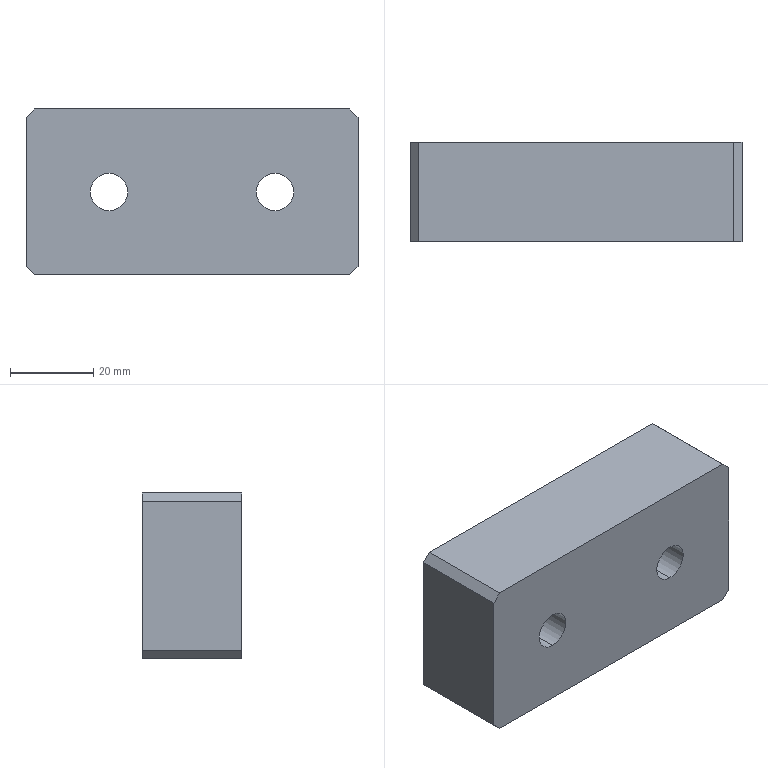Part | SolidWorks | features BaseBody 1 | 1 solid | 20 faces | box 80 x 24 x 40 mm | volume 71519 mm3 | plane 12 | cylinder 8 | commonest cylinder face diameters 9 x4 15 x4
STEP:
#1=CARTESIAN_POINT('',(-20.,15.,-7.5));
#2=VERTEX_POINT('',#1);
#3=CARTESIAN_POINT('',(-20.,15.,7.5));
#4=VERTEX_POINT('',#3);
#5=CARTESIAN_POINT('',(-20.,15.,0.));
#6=DIRECTION('',(0.,1.,0.));
#7=DIRECTION('',(0.,0.,1.));
#8=AXIS2_PLACEMENT_3D('',#5,#6,#7);
#9=CIRCLE('',#8,7.5);
#10=EDGE_CURVE('',#2,#4,#9,.T.);
#11=ORIENTED_EDGE('',*,*,#10,.F.);
#12=CARTESIAN_POINT('',(-20.,24.,-7.5));
#13=VERTEX_POINT('',#12);
#14=CARTESIAN_POINT('',(-20.,24.,-7.5));
#15=DIRECTION('',(0.,1.,0.));
#16=VECTOR('',#15,1000.);
#17=LINE('',#14,#16);
#18=EDGE_CURVE('',#2,#13,#17,.T.);
#19=ORIENTED_EDGE('',*,*,#18,.T.);
#20=CARTESIAN_POINT('',(-20.,24.,7.5));
#21=VERTEX_POINT('',#20);
#22=CARTESIAN_POINT('',(-20.,24.,0.));
#23=DIRECTION('',(0.,1.,0.));
#24=DIRECTION('',(0.,0.,1.));
#25=AXIS2_PLACEMENT_3D('',#22,#23,#24);
#26=CIRCLE('',#25,7.5);
#27=EDGE_CURVE('',#13,#21,#26,.T.);
#28=ORIENTED_EDGE('',*,*,#27,.T.);
#29=CARTESIAN_POINT('',(-20.,24.,7.5));
#30=DIRECTION('',(0.,1.,0.));
#31=VECTOR('',#30,1000.);
#32=LINE('',#29,#31);
#33=EDGE_CURVE('',#4,#21,#32,.T.);
#34=ORIENTED_EDGE('',*,*,#33,.F.);
#35=EDGE_LOOP('',(#11,#19,#28,#34));
#36=FACE_OUTER_BOUND('',#35,.T.);
#37=CARTESIAN_POINT('',(-20.,24.,0.));
#38=DIRECTION('',(0.,1.,0.));
#39=DIRECTION('',(0.,0.,1.));
#40=AXIS2_PLACEMENT_3D('',#37,#38,#39);
#41=CYLINDRICAL_SURFACE('',#40,7.5);
#42=ADVANCED_FACE('',(#36),#41,.F.);
#43=CARTESIAN_POINT('',(-20.,0.,-4.5));
#44=VERTEX_POINT('',#43);
#45=CARTESIAN_POINT('',(-20.,0.,4.5));
#46=VERTEX_POINT('',#45);
#47=CARTESIAN_POINT('',(-20.,0.,0.));
#48=DIRECTION('',(0.,1.,0.));
#49=DIRECTION('',(0.,0.,1.));
#50=AXIS2_PLACEMENT_3D('',#47,#48,#49);
#51=CIRCLE('',#50,4.5);
#52=EDGE_CURVE('',#44,#46,#51,.T.);
#53=ORIENTED_EDGE('',*,*,#52,.F.);
#54=CARTESIAN_POINT('',(-20.,15.,-4.5));
#55=VERTEX_POINT('',#54);
#56=CARTESIAN_POINT('',(-20.,24.,-4.5));
#57=DIRECTION('',(0.,1.,0.));
#58=VECTOR('',#57,1000.);
#59=LINE('',#56,#58);
#60=EDGE_CURVE('',#44,#55,#59,.T.);
#61=ORIENTED_EDGE('',*,*,#60,.T.);
#62=CARTESIAN_POINT('',(-20.,15.,4.5));
#63=VERTEX_POINT('',#62);
#64=CARTESIAN_POINT('',(-20.,15.,0.));
#65=DIRECTION('',(0.,1.,0.));
#66=DIRECTION('',(0.,0.,1.));
#67=AXIS2_PLACEMENT_3D('',#64,#65,#66);
#68=CIRCLE('',#67,4.5);
#69=EDGE_CURVE('',#55,#63,#68,.T.);
#70=ORIENTED_EDGE('',*,*,#69,.T.);
#71=CARTESIAN_POINT('',(-20.,24.,4.5));
#72=DIRECTION('',(0.,1.,0.));
#73=VECTOR('',#72,1000.);
#74=LINE('',#71,#73);
#75=EDGE_CURVE('',#46,#63,#74,.T.);
#76=ORIENTED_EDGE('',*,*,#75,.F.);
#77=EDGE_LOOP('',(#53,#61,#70,#76));
#78=FACE_OUTER_BOUND('',#77,.T.);
#79=CARTESIAN_POINT('',(-20.,24.,0.));
#80=DIRECTION('',(0.,1.,0.));
#81=DIRECTION('',(0.,0.,1.));
#82=AXIS2_PLACEMENT_3D('',#79,#80,#81);
#83=CYLINDRICAL_SURFACE('',#82,4.5);
#84=ADVANCED_FACE('',(#78),#83,.F.);
#85=CARTESIAN_POINT('',(20.,15.,-7.5));
#86=VERTEX_POINT('',#85);
#87=CARTESIAN_POINT('',(20.,15.,7.5));
#88=VERTEX_POINT('',#87);
#89=CARTESIAN_POINT('',(20.,15.,0.));
#90=DIRECTION('',(0.,1.,0.));
#91=DIRECTION('',(0.,0.,1.));
#92=AXIS2_PLACEMENT_3D('',#89,#90,#91);
#93=CIRCLE('',#92,7.5);
#94=EDGE_CURVE('',#86,#88,#93,.T.);
#95=ORIENTED_EDGE('',*,*,#94,.F.);
#96=CARTESIAN_POINT('',(20.,24.,-7.5));
#97=VERTEX_POINT('',#96);
#98=CARTESIAN_POINT('',(20.,24.,-7.5));
#99=DIRECTION('',(0.,1.,0.));
#100=VECTOR('',#99,1000.);
#101=LINE('',#98,#100);
#102=EDGE_CURVE('',#86,#97,#101,.T.);
#103=ORIENTED_EDGE('',*,*,#102,.T.);
#104=CARTESIAN_POINT('',(20.,24.,7.5));
#105=VERTEX_POINT('',#104);
#106=CARTESIAN_POINT('',(20.,24.,0.));
#107=DIRECTION('',(0.,1.,0.));
#108=DIRECTION('',(0.,0.,1.));
#109=AXIS2_PLACEMENT_3D('',#106,#107,#108);
#110=CIRCLE('',#109,7.5);
#111=EDGE_CURVE('',#97,#105,#110,.T.);
#112=ORIENTED_EDGE('',*,*,#111,.T.);
#113=CARTESIAN_POINT('',(20.,24.,7.5));
#114=DIRECTION('',(0.,1.,0.));
#115=VECTOR('',#114,1000.);
#116=LINE('',#113,#115);
#117=EDGE_CURVE('',#88,#105,#116,.T.);
#118=ORIENTED_EDGE('',*,*,#117,.F.);
#119=EDGE_LOOP('',(#95,#103,#112,#118));
#120=FACE_OUTER_BOUND('',#119,.T.);
#121=CARTESIAN_POINT('',(20.,24.,0.));
#122=DIRECTION('',(0.,1.,0.));
#123=DIRECTION('',(0.,0.,1.));
#124=AXIS2_PLACEMENT_3D('',#121,#122,#123);
#125=CYLINDRICAL_SURFACE('',#124,7.5);
#126=ADVANCED_FACE('',(#120),#125,.F.);
#127=CARTESIAN_POINT('',(20.,0.,-4.5));
#128=VERTEX_POINT('',#127);
#129=CARTESIAN_POINT('',(20.,0.,4.5));
#130=VERTEX_POINT('',#129);
#131=CARTESIAN_POINT('',(20.,0.,0.));
#132=DIRECTION('',(0.,1.,0.));
#133=DIRECTION('',(0.,0.,1.));
#134=AXIS2_PLACEMENT_3D('',#131,#132,#133);
#135=CIRCLE('',#134,4.5);
#136=EDGE_CURVE('',#128,#130,#135,.T.);
#137=ORIENTED_EDGE('',*,*,#136,.F.);
#138=CARTESIAN_POINT('',(20.,15.,-4.5));
#139=VERTEX_POINT('',#138);
#140=CARTESIAN_POINT('',(20.,24.,-4.5));
#141=DIRECTION('',(0.,1.,0.));
#142=VECTOR('',#141,1000.);
#143=LINE('',#140,#142);
#144=EDGE_CURVE('',#128,#139,#143,.T.);
#145=ORIENTED_EDGE('',*,*,#144,.T.);
#146=CARTESIAN_POINT('',(20.,15.,4.5));
#147=VERTEX_POINT('',#146);
#148=CARTESIAN_POINT('',(20.,15.,0.));
#149=DIRECTION('',(0.,1.,0.));
#150=DIRECTION('',(0.,0.,1.));
#151=AXIS2_PLACEMENT_3D('',#148,#149,#150);
#152=CIRCLE('',#151,4.5);
#153=EDGE_CURVE('',#139,#147,#152,.T.);
#154=ORIENTED_EDGE('',*,*,#153,.T.);
#155=CARTESIAN_POINT('',(20.,24.,4.5));
#156=DIRECTION('',(0.,1.,0.));
#157=VECTOR('',#156,1000.);
#158=LINE('',#155,#157);
#159=EDGE_CURVE('',#130,#147,#158,.T.);
#160=ORIENTED_EDGE('',*,*,#159,.F.);
#161=EDGE_LOOP('',(#137,#145,#154,#160));
#162=FACE_OUTER_BOUND('',#161,.T.);
#163=CARTESIAN_POINT('',(20.,24.,0.));
#164=DIRECTION('',(0.,1.,0.));
#165=DIRECTION('',(0.,0.,1.));
#166=AXIS2_PLACEMENT_3D('',#163,#164,#165);
#167=CYLINDRICAL_SURFACE('',#166,4.5);
#168=ADVANCED_FACE('',(#162),#167,.F.);
#169=CARTESIAN_POINT('',(-40.,24.,18.));
#170=VERTEX_POINT('',#169);
#171=CARTESIAN_POINT('',(-38.,24.,20.));
#172=VERTEX_POINT('',#171);
#173=CARTESIAN_POINT('',(-29.,24.,29.));
#174=DIRECTION('',(0.7071,0.,0.7071));
#175=VECTOR('',#174,1000.);
#176=LINE('',#173,#175);
#177=EDGE_CURVE('',#170,#172,#176,.T.);
#178=ORIENTED_EDGE('',*,*,#177,.F.);
#179=CARTESIAN_POINT('',(-40.,0.,18.));
#180=VERTEX_POINT('',#179);
#181=CARTESIAN_POINT('',(-40.,24.,18.));
#182=DIRECTION('',(0.,1.,0.));
#183=VECTOR('',#182,1000.);
#184=LINE('',#181,#183);
#185=EDGE_CURVE('',#180,#170,#184,.T.);
#186=ORIENTED_EDGE('',*,*,#185,.F.);
#187=CARTESIAN_POINT('',(-38.,0.,20.));
#188=VERTEX_POINT('',#187);
#189=CARTESIAN_POINT('',(-38.,0.,20.));
#190=DIRECTION('',(-0.7071,0.,-0.7071));
#191=VECTOR('',#190,1000.);
#192=LINE('',#189,#191);
#193=EDGE_CURVE('',#188,#180,#192,.T.);
#194=ORIENTED_EDGE('',*,*,#193,.F.);
#195=CARTESIAN_POINT('',(-38.,24.,20.));
#196=DIRECTION('',(0.,-1.,0.));
#197=VECTOR('',#196,1000.);
#198=LINE('',#195,#197);
#199=EDGE_CURVE('',#172,#188,#198,.T.);
#200=ORIENTED_EDGE('',*,*,#199,.F.);
#201=EDGE_LOOP('',(#178,#186,#194,#200));
#202=FACE_OUTER_BOUND('',#201,.T.);
#203=CARTESIAN_POINT('',(-38.,24.,20.));
#204=DIRECTION('',(0.7071,0.,-0.7071));
#205=DIRECTION('',(0.,-1.,0.));
#206=AXIS2_PLACEMENT_3D('',#203,#204,#205);
#207=PLANE('',#206);
#208=ADVANCED_FACE('',(#202),#207,.F.);
#209=CARTESIAN_POINT('',(-38.,24.,-20.));
#210=VERTEX_POINT('',#209);
#211=CARTESIAN_POINT('',(-40.,24.,-18.));
#212=VERTEX_POINT('',#211);
#213=CARTESIAN_POINT('',(-29.,24.,-29.));
#214=DIRECTION('',(-0.7071,0.,0.7071));
#215=VECTOR('',#214,1000.);
#216=LINE('',#213,#215);
#217=EDGE_CURVE('',#210,#212,#216,.T.);
#218=ORIENTED_EDGE('',*,*,#217,.F.);
#219=CARTESIAN_POINT('',(-38.,0.,-20.));
#220=VERTEX_POINT('',#219);
#221=CARTESIAN_POINT('',(-38.,24.,-20.));
#222=DIRECTION('',(0.,1.,0.));
#223=VECTOR('',#222,1000.);
#224=LINE('',#221,#223);
#225=EDGE_CURVE('',#220,#210,#224,.T.);
#226=ORIENTED_EDGE('',*,*,#225,.F.);
#227=CARTESIAN_POINT('',(-40.,0.,-18.));
#228=VERTEX_POINT('',#227);
#229=CARTESIAN_POINT('',(-40.,0.,-18.));
#230=DIRECTION('',(0.7071,0.,-0.7071));
#231=VECTOR('',#230,1000.);
#232=LINE('',#229,#231);
#233=EDGE_CURVE('',#228,#220,#232,.T.);
#234=ORIENTED_EDGE('',*,*,#233,.F.);
#235=CARTESIAN_POINT('',(-40.,24.,-18.));
#236=DIRECTION('',(0.,-1.,0.));
#237=VECTOR('',#236,1000.);
#238=LINE('',#235,#237);
#239=EDGE_CURVE('',#212,#228,#238,.T.);
#240=ORIENTED_EDGE('',*,*,#239,.F.);
#241=EDGE_LOOP('',(#218,#226,#234,#240));
#242=FACE_OUTER_BOUND('',#241,.T.);
#243=CARTESIAN_POINT('',(-40.,24.,-18.));
#244=DIRECTION('',(0.7071,0.,0.7071));
#245=DIRECTION('',(0.,-1.,0.));
#246=AXIS2_PLACEMENT_3D('',#243,#244,#245);
#247=PLANE('',#246);
#248=ADVANCED_FACE('',(#242),#247,.F.);
#249=CARTESIAN_POINT('',(38.,24.,20.));
#250=VERTEX_POINT('',#249);
#251=CARTESIAN_POINT('',(40.,24.,18.));
#252=VERTEX_POINT('',#251);
#253=CARTESIAN_POINT('',(29.,24.,29.));
#254=DIRECTION('',(0.7071,0.,-0.7071));
#255=VECTOR('',#254,1000.);
#256=LINE('',#253,#255);
#257=EDGE_CURVE('',#250,#252,#256,.T.);
#258=ORIENTED_EDGE('',*,*,#257,.F.);
#259=CARTESIAN_POINT('',(38.,0.,20.));
#260=VERTEX_POINT('',#259);
#261=CARTESIAN_POINT('',(38.,24.,20.));
#262=DIRECTION('',(0.,1.,0.));
#263=VECTOR('',#262,1000.);
#264=LINE('',#261,#263);
#265=EDGE_CURVE('',#260,#250,#264,.T.);
#266=ORIENTED_EDGE('',*,*,#265,.F.);
#267=CARTESIAN_POINT('',(40.,0.,18.));
#268=VERTEX_POINT('',#267);
#269=CARTESIAN_POINT('',(40.,0.,18.));
#270=DIRECTION('',(-0.7071,0.,0.7071));
#271=VECTOR('',#270,1000.);
#272=LINE('',#269,#271);
#273=EDGE_CURVE('',#268,#260,#272,.T.);
#274=ORIENTED_EDGE('',*,*,#273,.F.);
#275=CARTESIAN_POINT('',(40.,24.,18.));
#276=DIRECTION('',(0.,-1.,0.));
#277=VECTOR('',#276,1000.);
#278=LINE('',#275,#277);
#279=EDGE_CURVE('',#252,#268,#278,.T.);
#280=ORIENTED_EDGE('',*,*,#279,.F.);
#281=EDGE_LOOP('',(#258,#266,#274,#280));
#282=FACE_OUTER_BOUND('',#281,.T.);
#283=CARTESIAN_POINT('',(40.,24.,18.));
#284=DIRECTION('',(-0.7071,0.,-0.7071));
#285=DIRECTION('',(-0.7071,0.,0.7071));
#286=AXIS2_PLACEMENT_3D('',#283,#284,#285);
#287=PLANE('',#286);
#288=ADVANCED_FACE('',(#282),#287,.F.);
#289=CARTESIAN_POINT('',(40.,24.,-18.));
#290=VERTEX_POINT('',#289);
#291=CARTESIAN_POINT('',(38.,24.,-20.));
#292=VERTEX_POINT('',#291);
#293=CARTESIAN_POINT('',(29.,24.,-29.));
#294=DIRECTION('',(-0.7071,0.,-0.7071));
#295=VECTOR('',#294,1000.);
#296=LINE('',#293,#295);
#297=EDGE_CURVE('',#290,#292,#296,.T.);
#298=ORIENTED_EDGE('',*,*,#297,.F.);
#299=CARTESIAN_POINT('',(40.,0.,-18.));
#300=VERTEX_POINT('',#299);
#301=CARTESIAN_POINT('',(40.,24.,-18.));
#302=DIRECTION('',(0.,1.,0.));
#303=VECTOR('',#302,1000.);
#304=LINE('',#301,#303);
#305=EDGE_CURVE('',#300,#290,#304,.T.);
#306=ORIENTED_EDGE('',*,*,#305,.F.);
#307=CARTESIAN_POINT('',(38.,0.,-20.));
#308=VERTEX_POINT('',#307);
#309=CARTESIAN_POINT('',(38.,0.,-20.));
#310=DIRECTION('',(0.7071,0.,0.7071));
#311=VECTOR('',#310,1000.);
#312=LINE('',#309,#311);
#313=EDGE_CURVE('',#308,#300,#312,.T.);
#314=ORIENTED_EDGE('',*,*,#313,.F.);
#315=CARTESIAN_POINT('',(38.,24.,-20.));
#316=DIRECTION('',(0.,-1.,0.));
#317=VECTOR('',#316,1000.);
#318=LINE('',#315,#317);
#319=EDGE_CURVE('',#292,#308,#318,.T.);
#320=ORIENTED_EDGE('',*,*,#319,.F.);
#321=EDGE_LOOP('',(#298,#306,#314,#320));
#322=FACE_OUTER_BOUND('',#321,.T.);
#323=CARTESIAN_POINT('',(38.,24.,-20.));
#324=DIRECTION('',(-0.7071,0.,0.7071));
#325=DIRECTION('',(0.,1.,0.));
#326=AXIS2_PLACEMENT_3D('',#323,#324,#325);
#327=PLANE('',#326);
#328=ADVANCED_FACE('',(#322),#327,.F.);
#329=CARTESIAN_POINT('',(-20.,15.,0.));
#330=DIRECTION('',(0.,1.,0.));
#331=DIRECTION('',(0.,0.,1.));
#332=AXIS2_PLACEMENT_3D('',#329,#330,#331);
#333=CIRCLE('',#332,4.5);
#334=EDGE_CURVE('',#63,#55,#333,.T.);
#335=ORIENTED_EDGE('',*,*,#334,.F.);
#336=ORIENTED_EDGE('',*,*,#69,.F.);
#337=EDGE_LOOP('',(#335,#336));
#338=FACE_BOUND('',#337,.T.);
#339=CARTESIAN_POINT('',(-20.,15.,0.));
#340=DIRECTION('',(0.,1.,0.));
#341=DIRECTION('',(0.,0.,1.));
#342=AXIS2_PLACEMENT_3D('',#339,#340,#341);
#343=CIRCLE('',#342,7.5);
#344=EDGE_CURVE('',#4,#2,#343,.T.);
#345=ORIENTED_EDGE('',*,*,#344,.T.);
#346=ORIENTED_EDGE('',*,*,#10,.T.);
#347=EDGE_LOOP('',(#345,#346));
#348=FACE_OUTER_BOUND('',#347,.T.);
#349=CARTESIAN_POINT('',(-15.5,15.,0.));
#350=DIRECTION('',(0.,-1.,0.));
#351=DIRECTION('',(0.,0.,-1.));
#352=AXIS2_PLACEMENT_3D('',#349,#350,#351);
#353=PLANE('',#352);
#354=ADVANCED_FACE('',(#338,#348),#353,.F.);
#355=CARTESIAN_POINT('',(20.,15.,0.));
#356=DIRECTION('',(0.,1.,0.));
#357=DIRECTION('',(0.,0.,1.));
#358=AXIS2_PLACEMENT_3D('',#355,#356,#357);
#359=CIRCLE('',#358,4.5);
#360=EDGE_CURVE('',#147,#139,#359,.T.);
#361=ORIENTED_EDGE('',*,*,#360,.F.);
#362=ORIENTED_EDGE('',*,*,#153,.F.);
#363=EDGE_LOOP('',(#361,#362));
#364=FACE_BOUND('',#363,.T.);
#365=CARTESIAN_POINT('',(20.,15.,0.));
#366=DIRECTION('',(0.,1.,0.));
#367=DIRECTION('',(0.,0.,1.));
#368=AXIS2_PLACEMENT_3D('',#365,#366,#367);
#369=CIRCLE('',#368,7.5);
#370=EDGE_CURVE('',#88,#86,#369,.T.);
#371=ORIENTED_EDGE('',*,*,#370,.T.);
#372=ORIENTED_EDGE('',*,*,#94,.T.);
#373=EDGE_LOOP('',(#371,#372));
#374=FACE_OUTER_BOUND('',#373,.T.);
#375=CARTESIAN_POINT('',(24.5,15.,0.));
#376=DIRECTION('',(0.,-1.,0.));
#377=DIRECTION('',(0.,0.,-1.));
#378=AXIS2_PLACEMENT_3D('',#375,#376,#377);
#379=PLANE('',#378);
#380=ADVANCED_FACE('',(#364,#374),#379,.F.);
#381=CARTESIAN_POINT('',(20.,0.,0.));
#382=DIRECTION('',(0.,1.,0.));
#383=DIRECTION('',(0.,0.,1.));
#384=AXIS2_PLACEMENT_3D('',#381,#382,#383);
#385=CIRCLE('',#384,4.5);
#386=EDGE_CURVE('',#130,#128,#385,.T.);
#387=ORIENTED_EDGE('',*,*,#386,.T.);
#388=ORIENTED_EDGE('',*,*,#136,.T.);
#389=EDGE_LOOP('',(#387,#388));
#390=FACE_BOUND('',#389,.T.);
#391=CARTESIAN_POINT('',(-20.,0.,0.));
#392=DIRECTION('',(0.,1.,0.));
#393=DIRECTION('',(0.,0.,1.));
#394=AXIS2_PLACEMENT_3D('',#391,#392,#393);
#395=CIRCLE('',#394,4.5);
#396=EDGE_CURVE('',#46,#44,#395,.T.);
#397=ORIENTED_EDGE('',*,*,#396,.T.);
#398=ORIENTED_EDGE('',*,*,#52,.T.);
#399=EDGE_LOOP('',(#397,#398));
#400=FACE_BOUND('',#399,.T.);
#401=CARTESIAN_POINT('',(-40.,0.,-20.));
#402=DIRECTION('',(-1.,0.,0.));
#403=VECTOR('',#402,1000.);
#404=LINE('',#401,#403);
#405=EDGE_CURVE('',#308,#220,#404,.T.);
#406=ORIENTED_EDGE('',*,*,#405,.F.);
#407=ORIENTED_EDGE('',*,*,#313,.T.);
#408=CARTESIAN_POINT('',(40.,0.,-20.));
#409=DIRECTION('',(0.,0.,-1.));
#410=VECTOR('',#409,1000.);
#411=LINE('',#408,#410);
#412=EDGE_CURVE('',#268,#300,#411,.T.);
#413=ORIENTED_EDGE('',*,*,#412,.F.);
#414=ORIENTED_EDGE('',*,*,#273,.T.);
#415=CARTESIAN_POINT('',(-40.,0.,20.));
#416=DIRECTION('',(1.,0.,0.));
#417=VECTOR('',#416,1000.);
#418=LINE('',#415,#417);
#419=EDGE_CURVE('',#188,#260,#418,.T.);
#420=ORIENTED_EDGE('',*,*,#419,.F.);
#421=ORIENTED_EDGE('',*,*,#193,.T.);
#422=CARTESIAN_POINT('',(-40.,0.,-20.));
#423=DIRECTION('',(0.,0.,1.));
#424=VECTOR('',#423,1000.);
#425=LINE('',#422,#424);
#426=EDGE_CURVE('',#228,#180,#425,.T.);
#427=ORIENTED_EDGE('',*,*,#426,.F.);
#428=ORIENTED_EDGE('',*,*,#233,.T.);
#429=EDGE_LOOP('',(#406,#407,#413,#414,#420,#421,#427,#428));
#430=FACE_OUTER_BOUND('',#429,.T.);
#431=CARTESIAN_POINT('',(0.,0.,0.));
#432=DIRECTION('',(0.,1.,0.));
#433=DIRECTION('',(1.,0.,0.));
#434=AXIS2_PLACEMENT_3D('',#431,#432,#433);
#435=PLANE('',#434);
#436=ADVANCED_FACE('',(#390,#400,#430),#435,.F.);
#437=CARTESIAN_POINT('',(20.,24.,0.));
#438=DIRECTION('',(0.,1.,0.));
#439=DIRECTION('',(0.,0.,1.));
#440=AXIS2_PLACEMENT_3D('',#437,#438,#439);
#441=CIRCLE('',#440,7.5);
#442=EDGE_CURVE('',#105,#97,#441,.T.);
#443=ORIENTED_EDGE('',*,*,#442,.F.);
#444=ORIENTED_EDGE('',*,*,#111,.F.);
#445=EDGE_LOOP('',(#443,#444));
#446=FACE_BOUND('',#445,.T.);
#447=CARTESIAN_POINT('',(-20.,24.,0.));
#448=DIRECTION('',(0.,1.,0.));
#449=DIRECTION('',(0.,0.,1.));
#450=AXIS2_PLACEMENT_3D('',#447,#448,#449);
#451=CIRCLE('',#450,7.5);
#452=EDGE_CURVE('',#21,#13,#451,.T.);
#453=ORIENTED_EDGE('',*,*,#452,.F.);
#454=ORIENTED_EDGE('',*,*,#27,.F.);
#455=EDGE_LOOP('',(#453,#454));
#456=FACE_BOUND('',#455,.T.);
#457=CARTESIAN_POINT('',(40.,24.,-20.));
#458=DIRECTION('',(0.,0.,-1.));
#459=VECTOR('',#458,1000.);
#460=LINE('',#457,#459);
#461=EDGE_CURVE('',#252,#290,#460,.T.);
#462=ORIENTED_EDGE('',*,*,#461,.T.);
#463=ORIENTED_EDGE('',*,*,#297,.T.);
#464=CARTESIAN_POINT('',(-40.,24.,-20.));
#465=DIRECTION('',(-1.,0.,0.));
#466=VECTOR('',#465,1000.);
#467=LINE('',#464,#466);
#468=EDGE_CURVE('',#292,#210,#467,.T.);
#469=ORIENTED_EDGE('',*,*,#468,.T.);
#470=ORIENTED_EDGE('',*,*,#217,.T.);
#471=CARTESIAN_POINT('',(-40.,24.,-20.));
#472=DIRECTION('',(0.,0.,1.));
#473=VECTOR('',#472,1000.);
#474=LINE('',#471,#473);
#475=EDGE_CURVE('',#212,#170,#474,.T.);
#476=ORIENTED_EDGE('',*,*,#475,.T.);
#477=ORIENTED_EDGE('',*,*,#177,.T.);
#478=CARTESIAN_POINT('',(-40.,24.,20.));
#479=DIRECTION('',(1.,0.,0.));
#480=VECTOR('',#479,1000.);
#481=LINE('',#478,#480);
#482=EDGE_CURVE('',#172,#250,#481,.T.);
#483=ORIENTED_EDGE('',*,*,#482,.T.);
#484=ORIENTED_EDGE('',*,*,#257,.T.);
#485=EDGE_LOOP('',(#462,#463,#469,#470,#476,#477,#483,#484));
#486=FACE_OUTER_BOUND('',#485,.T.);
#487=CARTESIAN_POINT('',(0.,24.,0.));
#488=DIRECTION('',(0.,1.,0.));
#489=DIRECTION('',(1.,0.,0.));
#490=AXIS2_PLACEMENT_3D('',#487,#488,#489);
#491=PLANE('',#490);
#492=ADVANCED_FACE('',(#446,#456,#486),#491,.T.);
#493=ORIENTED_EDGE('',*,*,#419,.T.);
#494=ORIENTED_EDGE('',*,*,#265,.T.);
#495=ORIENTED_EDGE('',*,*,#482,.F.);
#496=ORIENTED_EDGE('',*,*,#199,.T.);
#497=EDGE_LOOP('',(#493,#494,#495,#496));
#498=FACE_OUTER_BOUND('',#497,.T.);
#499=CARTESIAN_POINT('',(-40.,24.,20.));
#500=DIRECTION('',(0.,0.,-1.));
#501=DIRECTION('',(0.,-1.,0.));
#502=AXIS2_PLACEMENT_3D('',#499,#500,#501);
#503=PLANE('',#502);
#504=ADVANCED_FACE('',(#498),#503,.F.);
#505=ORIENTED_EDGE('',*,*,#475,.F.);
#506=ORIENTED_EDGE('',*,*,#239,.T.);
#507=ORIENTED_EDGE('',*,*,#426,.T.);
#508=ORIENTED_EDGE('',*,*,#185,.T.);
#509=EDGE_LOOP('',(#505,#506,#507,#508));
#510=FACE_OUTER_BOUND('',#509,.T.);
#511=CARTESIAN_POINT('',(-40.,24.,-20.));
#512=DIRECTION('',(1.,0.,0.));
#513=DIRECTION('',(0.,1.,0.));
#514=AXIS2_PLACEMENT_3D('',#511,#512,#513);
#515=PLANE('',#514);
#516=ADVANCED_FACE('',(#510),#515,.F.);
#517=ORIENTED_EDGE('',*,*,#468,.F.);
#518=ORIENTED_EDGE('',*,*,#319,.T.);
#519=ORIENTED_EDGE('',*,*,#405,.T.);
#520=ORIENTED_EDGE('',*,*,#225,.T.);
#521=EDGE_LOOP('',(#517,#518,#519,#520));
#522=FACE_OUTER_BOUND('',#521,.T.);
#523=CARTESIAN_POINT('',(-40.,24.,-20.));
#524=DIRECTION('',(0.,0.,1.));
#525=DIRECTION('',(1.,0.,0.));
#526=AXIS2_PLACEMENT_3D('',#523,#524,#525);
#527=PLANE('',#526);
#528=ADVANCED_FACE('',(#522),#527,.F.);
#529=ORIENTED_EDGE('',*,*,#412,.T.);
#530=ORIENTED_EDGE('',*,*,#305,.T.);
#531=ORIENTED_EDGE('',*,*,#461,.F.);
#532=ORIENTED_EDGE('',*,*,#279,.T.);
#533=EDGE_LOOP('',(#529,#530,#531,#532));
#534=FACE_OUTER_BOUND('',#533,.T.);
#535=CARTESIAN_POINT('',(40.,24.,-20.));
#536=DIRECTION('',(-1.,0.,0.));
#537=DIRECTION('',(0.,1.,0.));
#538=AXIS2_PLACEMENT_3D('',#535,#536,#537);
#539=PLANE('',#538);
#540=ADVANCED_FACE('',(#534),#539,.F.);
#541=ORIENTED_EDGE('',*,*,#144,.F.);
#542=ORIENTED_EDGE('',*,*,#386,.F.);
#543=ORIENTED_EDGE('',*,*,#159,.T.);
#544=ORIENTED_EDGE('',*,*,#360,.T.);
#545=EDGE_LOOP('',(#541,#542,#543,#544));
#546=FACE_OUTER_BOUND('',#545,.T.);
#547=CARTESIAN_POINT('',(20.,24.,0.));
#548=DIRECTION('',(0.,1.,0.));
#549=DIRECTION('',(0.,0.,1.));
#550=AXIS2_PLACEMENT_3D('',#547,#548,#549);
#551=CYLINDRICAL_SURFACE('',#550,4.5);
#552=ADVANCED_FACE('',(#546),#551,.F.);
#553=ORIENTED_EDGE('',*,*,#102,.F.);
#554=ORIENTED_EDGE('',*,*,#370,.F.);
#555=ORIENTED_EDGE('',*,*,#117,.T.);
#556=ORIENTED_EDGE('',*,*,#442,.T.);
#557=EDGE_LOOP('',(#553,#554,#555,#556));
#558=FACE_OUTER_BOUND('',#557,.T.);
#559=CARTESIAN_POINT('',(20.,24.,0.));
#560=DIRECTION('',(0.,1.,0.));
#561=DIRECTION('',(0.,0.,1.));
#562=AXIS2_PLACEMENT_3D('',#559,#560,#561);
#563=CYLINDRICAL_SURFACE('',#562,7.5);
#564=ADVANCED_FACE('',(#558),#563,.F.);
#565=ORIENTED_EDGE('',*,*,#60,.F.);
#566=ORIENTED_EDGE('',*,*,#396,.F.);
#567=ORIENTED_EDGE('',*,*,#75,.T.);
#568=ORIENTED_EDGE('',*,*,#334,.T.);
#569=EDGE_LOOP('',(#565,#566,#567,#568));
#570=FACE_OUTER_BOUND('',#569,.T.);
#571=CARTESIAN_POINT('',(-20.,24.,0.));
#572=DIRECTION('',(0.,1.,0.));
#573=DIRECTION('',(0.,0.,1.));
#574=AXIS2_PLACEMENT_3D('',#571,#572,#573);
#575=CYLINDRICAL_SURFACE('',#574,4.5);
#576=ADVANCED_FACE('',(#570),#575,.F.);
#577=ORIENTED_EDGE('',*,*,#18,.F.);
#578=ORIENTED_EDGE('',*,*,#344,.F.);
#579=ORIENTED_EDGE('',*,*,#33,.T.);
#580=ORIENTED_EDGE('',*,*,#452,.T.);
#581=EDGE_LOOP('',(#577,#578,#579,#580));
#582=FACE_OUTER_BOUND('',#581,.T.);
#583=CARTESIAN_POINT('',(-20.,24.,0.));
#584=DIRECTION('',(0.,1.,0.));
#585=DIRECTION('',(0.,0.,1.));
#586=AXIS2_PLACEMENT_3D('',#583,#584,#585);
#587=CYLINDRICAL_SURFACE('',#586,7.5);
#588=ADVANCED_FACE('',(#582),#587,.F.);
#589=CLOSED_SHELL('',(#42,#84,#126,#168,#208,#248,#288,#328,#354,#380,#436,#492,#504,#516,#528,#540,#552,#564,#576,#588));
#590=MANIFOLD_SOLID_BREP('',#589);
#591=CARTESIAN_POINT('',(0.,0.,0.));
#592=DIRECTION('',(0.,0.,1.));
#593=DIRECTION('',(1.,0.,0.));
#594=AXIS2_PLACEMENT_3D('',#591,#592,#593);
#595=(LENGTH_UNIT()NAMED_UNIT(*)SI_UNIT(.MILLI.,.METRE.));
#596=UNCERTAINTY_MEASURE_WITH_UNIT(LENGTH_MEASURE(0.00001),#595,'','');
#597=(NAMED_UNIT(*)PLANE_ANGLE_UNIT()SI_UNIT($,.RADIAN.));
#598=(NAMED_UNIT(*)SI_UNIT($,.STERADIAN.)SOLID_ANGLE_UNIT());
#599=(GEOMETRIC_REPRESENTATION_CONTEXT(3)GLOBAL_UNCERTAINTY_ASSIGNED_CONTEXT((#596))GLOBAL_UNIT_ASSIGNED_CONTEXT((#595,#597,#598))REPRESENTATION_CONTEXT('',''));
#600=ADVANCED_BREP_SHAPE_REPRESENTATION('',(#590,#594),#599);